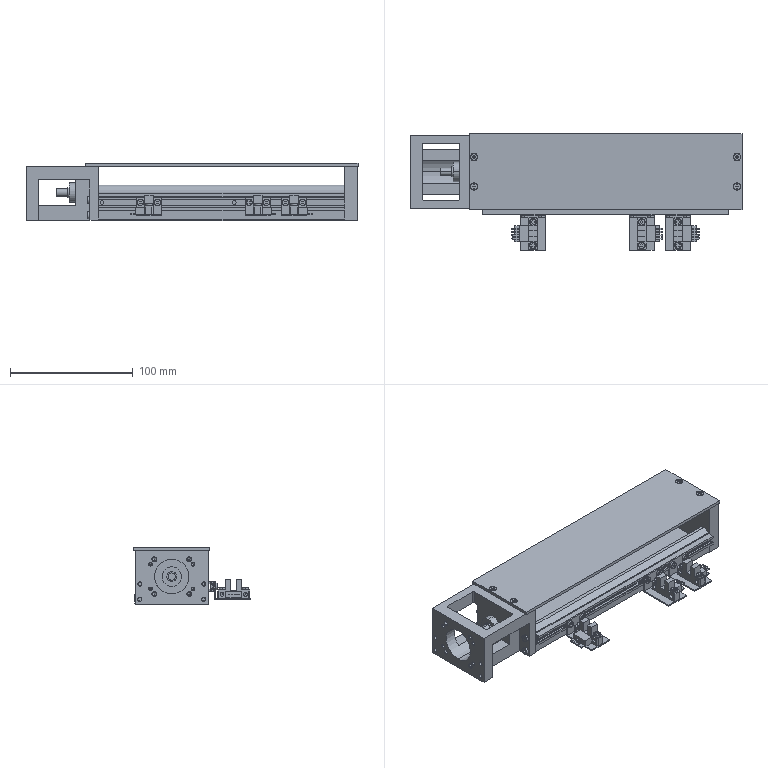Part | STEP file | PRODUCT_ID_1-C-F0-200 | 1 solid | 929 faces | box 270.02 x 94.86 x 47 mm | volume 309343 mm3 | plane 527 | cylinder 236 | cone 126 | spline 40 | commonest cylinder face diameters 5.5 x48 3.19 x24 1.2 x20 2 x20 3.21 x18 2.459 x16